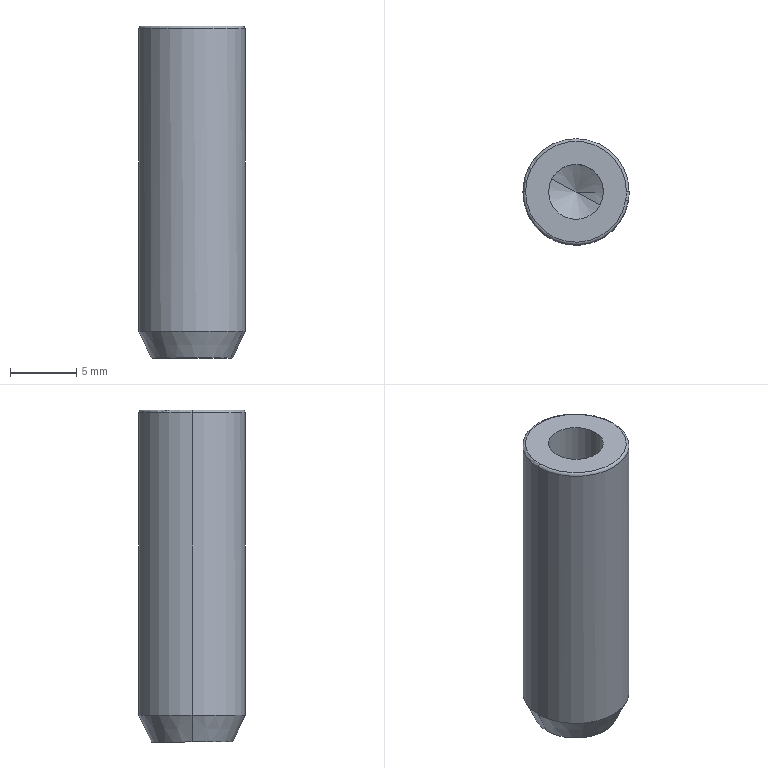Part | CATIA | 1 solid | 14 faces | box 8 x 8 x 25 mm | volume 1095 mm3 | cone 5 | cylinder 4 | torus 3 | plane 2 | commonest cylinder face diameters 4.134 x2 8 x2
STEP:
#1=CARTESIAN_POINT('',(0.,0.,13.807));
#2=VERTEX_POINT('',#1);
#3=CARTESIAN_POINT('',(-1.814,0.991,15.));
#4=VERTEX_POINT('',#3);
#5=CARTESIAN_POINT('',(-380004.396,207597.348,250013.807));
#6=DIRECTION('',(-0.76,0.4152,0.5));
#7=VECTOR('',#6,1.);
#8=LINE('',#5,#7);
#9=EDGE_CURVE('',#2,#4,#8,.T.);
#10=ORIENTED_EDGE('',*,*,#9,.T.);
#11=CARTESIAN_POINT('',(1.814,-0.991,15.));
#12=VERTEX_POINT('',#11);
#13=CARTESIAN_POINT('',(0.,0.,15.));
#14=DIRECTION('',(0.,0.,1.));
#15=AXIS2_PLACEMENT_3D('',#13,#14,$);
#16=CIRCLE('',#15,2.067);
#17=EDGE_CURVE('',#12,#4,#16,.F.);
#18=ORIENTED_EDGE('',*,*,#17,.F.);
#19=CARTESIAN_POINT('',(380004.396,-207597.348,250013.807));
#20=DIRECTION('',(0.76,-0.4152,0.5));
#21=VECTOR('',#20,1.);
#22=LINE('',#19,#21);
#23=EDGE_CURVE('',#2,#12,#22,.T.);
#24=ORIENTED_EDGE('',*,*,#23,.F.);
#25=EDGE_LOOP('',(#10,#18,#24));
#26=FACE_OUTER_BOUND('',#25,.T.);
#27=CARTESIAN_POINT('',(0.,0.,13.807));
#28=DIRECTION('',(0.,0.,1.));
#29=DIRECTION('',(-0.8776,0.4794,0.));
#30=AXIS2_PLACEMENT_3D('',#27,#28,#29);
#31=CONICAL_SURFACE('',#30,0.,1.047);
#32=ADVANCED_FACE('',(#26),#31,.F.);
#33=ORIENTED_EDGE('',*,*,#23,.T.);
#34=CARTESIAN_POINT('',(0.,0.,15.));
#35=DIRECTION('',(0.,0.,1.));
#36=AXIS2_PLACEMENT_3D('',#34,#35,$);
#37=CIRCLE('',#36,2.067);
#38=EDGE_CURVE('',#4,#12,#37,.F.);
#39=ORIENTED_EDGE('',*,*,#38,.F.);
#40=ORIENTED_EDGE('',*,*,#9,.F.);
#41=EDGE_LOOP('',(#33,#39,#40));
#42=FACE_OUTER_BOUND('',#41,.T.);
#43=CARTESIAN_POINT('',(0.,0.,13.807));
#44=DIRECTION('',(0.,0.,1.));
#45=DIRECTION('',(0.8776,-0.4794,0.));
#46=AXIS2_PLACEMENT_3D('',#43,#44,#45);
#47=CONICAL_SURFACE('',#46,0.,1.047);
#48=ADVANCED_FACE('',(#42),#47,.F.);
#49=CARTESIAN_POINT('',(-1.814,0.991,25.));
#50=VERTEX_POINT('',#49);
#51=CARTESIAN_POINT('',(1.814,-0.991,25.));
#52=VERTEX_POINT('',#51);
#53=CARTESIAN_POINT('',(0.,0.,25.));
#54=DIRECTION('',(0.,0.,-1.));
#55=AXIS2_PLACEMENT_3D('',#53,#54,$);
#56=CIRCLE('',#55,2.067);
#57=EDGE_CURVE('',#50,#52,#56,.F.);
#58=ORIENTED_EDGE('',*,*,#57,.T.);
#59=CARTESIAN_POINT('',(1.814,-0.991,24.9));
#60=DIRECTION('',(0.,0.,-1.));
#61=VECTOR('',#60,1.);
#62=LINE('',#59,#61);
#63=EDGE_CURVE('',#12,#52,#62,.F.);
#64=ORIENTED_EDGE('',*,*,#63,.F.);
#65=ORIENTED_EDGE('',*,*,#17,.T.);
#66=CARTESIAN_POINT('',(-1.814,0.991,24.9));
#67=DIRECTION('',(0.,0.,-1.));
#68=VECTOR('',#67,1.);
#69=LINE('',#66,#68);
#70=EDGE_CURVE('',#4,#50,#69,.F.);
#71=ORIENTED_EDGE('',*,*,#70,.T.);
#72=EDGE_LOOP('',(#58,#64,#65,#71));
#73=FACE_OUTER_BOUND('',#72,.T.);
#74=CARTESIAN_POINT('',(0.,0.,24.9));
#75=DIRECTION('',(0.,0.,-1.));
#76=DIRECTION('',(0.8776,-0.4794,0.));
#77=AXIS2_PLACEMENT_3D('',#74,#75,#76);
#78=CYLINDRICAL_SURFACE('',#77,2.067);
#79=ADVANCED_FACE('',(#73),#78,.F.);
#80=CARTESIAN_POINT('',(1.814,-0.991,25.));
#81=CARTESIAN_POINT('',(2.125,-0.4211,25.));
#82=CARTESIAN_POINT('',(2.213,0.271,25.));
#83=CARTESIAN_POINT('',(2.008,0.9675,25.));
#84=CARTESIAN_POINT('',(1.113,2.038,25.));
#85=CARTESIAN_POINT('',(-0.271,2.213,25.));
#86=CARTESIAN_POINT('',(-0.9675,2.008,25.));
#87=CARTESIAN_POINT('',(-1.503,1.561,25.));
#88=CARTESIAN_POINT('',(-1.814,0.991,25.));
#89=B_SPLINE_CURVE_WITH_KNOTS('',5,(#80,#81,#82,#83,#84,#85,#86,#87,#88),.UNSPECIFIED.,.F.,.U.,(6,3,6),(-3.247,0.,3.247),.UNSPECIFIED.);
#90=EDGE_CURVE('',#52,#50,#89,.T.);
#91=ORIENTED_EDGE('',*,*,#90,.T.);
#92=ORIENTED_EDGE('',*,*,#70,.F.);
#93=ORIENTED_EDGE('',*,*,#38,.T.);
#94=ORIENTED_EDGE('',*,*,#63,.T.);
#95=EDGE_LOOP('',(#91,#92,#93,#94));
#96=FACE_OUTER_BOUND('',#95,.T.);
#97=CARTESIAN_POINT('',(0.,0.,24.9));
#98=DIRECTION('',(0.,0.,-1.));
#99=DIRECTION('',(-0.8776,0.4794,0.));
#100=AXIS2_PLACEMENT_3D('',#97,#98,#99);
#101=CYLINDRICAL_SURFACE('',#100,2.067);
#102=ADVANCED_FACE('',(#96),#101,.F.);
#103=CARTESIAN_POINT('',(-3.8,0.000000372,25.));
#104=VERTEX_POINT('',#103);
#105=CARTESIAN_POINT('',(3.75,-0.6142,25.));
#106=VERTEX_POINT('',#105);
#107=CARTESIAN_POINT('',(0.,0.,25.));
#108=DIRECTION('',(0.,0.,1.));
#109=AXIS2_PLACEMENT_3D('',#107,#108,$);
#110=CIRCLE('',#109,3.8);
#111=EDGE_CURVE('',#104,#106,#110,.T.);
#112=ORIENTED_EDGE('',*,*,#111,.T.);
#113=CARTESIAN_POINT('',(3.8,0.,25.));
#114=VERTEX_POINT('',#113);
#115=CARTESIAN_POINT('',(0.,0.,25.));
#116=DIRECTION('',(0.,0.,1.));
#117=AXIS2_PLACEMENT_3D('',#115,#116,$);
#118=CIRCLE('',#117,3.8);
#119=EDGE_CURVE('',#106,#114,#118,.T.);
#120=ORIENTED_EDGE('',*,*,#119,.T.);
#121=CARTESIAN_POINT('',(0.,0.,25.));
#122=DIRECTION('',(0.,0.,1.));
#123=AXIS2_PLACEMENT_3D('',#121,#122,$);
#124=CIRCLE('',#123,3.8);
#125=EDGE_CURVE('',#114,#104,#124,.T.);
#126=ORIENTED_EDGE('',*,*,#125,.T.);
#127=EDGE_LOOP('',(#112,#120,#126));
#128=FACE_OUTER_BOUND('',#127,.T.);
#129=ORIENTED_EDGE('',*,*,#57,.F.);
#130=ORIENTED_EDGE('',*,*,#90,.F.);
#131=EDGE_LOOP('',(#129,#130));
#132=FACE_BOUND('',#131,.T.);
#133=CARTESIAN_POINT('',(0.,0.,25.));
#134=DIRECTION('',(0.,0.,1.));
#135=DIRECTION('',(1.,0.,0.));
#136=AXIS2_PLACEMENT_3D('',#133,#134,#135);
#137=PLANE('',#136);
#138=ADVANCED_FACE('',(#128,#132),#137,.T.);
#139=CARTESIAN_POINT('',(3.947,-0.6465,24.8));
#140=VERTEX_POINT('',#139);
#141=CARTESIAN_POINT('',(3.75,-0.6142,24.8));
#142=DIRECTION('',(-0.1616,-0.9869,0.));
#143=AXIS2_PLACEMENT_3D('',#141,#142,$);
#144=CIRCLE('',#143,0.2);
#145=EDGE_CURVE('',#140,#106,#144,.T.);
#146=ORIENTED_EDGE('',*,*,#145,.T.);
#147=ORIENTED_EDGE('',*,*,#111,.F.);
#148=CARTESIAN_POINT('',(-4.,0.,24.8));
#149=VERTEX_POINT('',#148);
#150=CARTESIAN_POINT('',(-3.8,0.,24.8));
#151=DIRECTION('',(0.,1.,0.));
#152=AXIS2_PLACEMENT_3D('',#150,#151,$);
#153=CIRCLE('',#152,0.2);
#154=EDGE_CURVE('',#104,#149,#153,.F.);
#155=ORIENTED_EDGE('',*,*,#154,.T.);
#156=CARTESIAN_POINT('',(0.,0.,24.8));
#157=DIRECTION('',(0.,0.,1.));
#158=AXIS2_PLACEMENT_3D('',#156,#157,$);
#159=CIRCLE('',#158,4.);
#160=EDGE_CURVE('',#149,#140,#159,.T.);
#161=ORIENTED_EDGE('',*,*,#160,.T.);
#162=EDGE_LOOP('',(#146,#147,#155,#161));
#163=FACE_OUTER_BOUND('',#162,.T.);
#164=CARTESIAN_POINT('',(0.,0.,24.8));
#165=DIRECTION('',(0.,0.,1.));
#166=DIRECTION('',(-0.9869,0.1616,0.));
#167=AXIS2_PLACEMENT_3D('',#164,#165,#166);
#168=TOROIDAL_SURFACE('',#167,3.8,0.2);
#169=ADVANCED_FACE('',(#163),#168,.T.);
#170=ORIENTED_EDGE('',*,*,#145,.F.);
#171=CARTESIAN_POINT('',(4.,0.,24.8));
#172=VERTEX_POINT('',#171);
#173=CARTESIAN_POINT('',(0.,0.,24.8));
#174=DIRECTION('',(0.,0.,1.));
#175=AXIS2_PLACEMENT_3D('',#173,#174,$);
#176=CIRCLE('',#175,4.);
#177=EDGE_CURVE('',#140,#172,#176,.T.);
#178=ORIENTED_EDGE('',*,*,#177,.T.);
#179=CARTESIAN_POINT('',(3.8,0.,24.8));
#180=DIRECTION('',(0.,-1.,0.));
#181=AXIS2_PLACEMENT_3D('',#179,#180,$);
#182=CIRCLE('',#181,0.2);
#183=EDGE_CURVE('',#114,#172,#182,.F.);
#184=ORIENTED_EDGE('',*,*,#183,.F.);
#185=ORIENTED_EDGE('',*,*,#119,.F.);
#186=EDGE_LOOP('',(#170,#178,#184,#185));
#187=FACE_OUTER_BOUND('',#186,.T.);
#188=CARTESIAN_POINT('',(0.,0.,24.8));
#189=DIRECTION('',(0.,0.,1.));
#190=DIRECTION('',(0.9869,-0.1616,0.));
#191=AXIS2_PLACEMENT_3D('',#188,#189,#190);
#192=TOROIDAL_SURFACE('',#191,3.8,0.2);
#193=ADVANCED_FACE('',(#187),#192,.T.);
#194=ORIENTED_EDGE('',*,*,#183,.T.);
#195=CARTESIAN_POINT('',(0.,0.,24.8));
#196=DIRECTION('',(0.,0.,1.));
#197=AXIS2_PLACEMENT_3D('',#195,#196,$);
#198=CIRCLE('',#197,4.);
#199=EDGE_CURVE('',#172,#149,#198,.T.);
#200=ORIENTED_EDGE('',*,*,#199,.T.);
#201=ORIENTED_EDGE('',*,*,#154,.F.);
#202=ORIENTED_EDGE('',*,*,#125,.F.);
#203=EDGE_LOOP('',(#194,#200,#201,#202));
#204=FACE_OUTER_BOUND('',#203,.T.);
#205=CARTESIAN_POINT('',(0.,0.,24.8));
#206=DIRECTION('',(0.,0.,1.));
#207=DIRECTION('',(1.,0.,0.));
#208=AXIS2_PLACEMENT_3D('',#205,#206,#207);
#209=TOROIDAL_SURFACE('',#208,3.8,0.2);
#210=ADVANCED_FACE('',(#204),#209,.T.);
#211=CARTESIAN_POINT('',(4.,0.,2.));
#212=VERTEX_POINT('',#211);
#213=CARTESIAN_POINT('',(4.,0.,12.5));
#214=DIRECTION('',(0.,0.,1.));
#215=VECTOR('',#214,1.);
#216=LINE('',#213,#215);
#217=EDGE_CURVE('',#212,#172,#216,.T.);
#218=ORIENTED_EDGE('',*,*,#217,.T.);
#219=ORIENTED_EDGE('',*,*,#177,.F.);
#220=ORIENTED_EDGE('',*,*,#160,.F.);
#221=CARTESIAN_POINT('',(-4.,0.,2.));
#222=VERTEX_POINT('',#221);
#223=CARTESIAN_POINT('',(-4.,0.,12.5));
#224=DIRECTION('',(0.,0.,1.));
#225=VECTOR('',#224,1.);
#226=LINE('',#223,#225);
#227=EDGE_CURVE('',#222,#149,#226,.T.);
#228=ORIENTED_EDGE('',*,*,#227,.F.);
#229=CARTESIAN_POINT('',(3.787,-1.287,2.));
#230=VERTEX_POINT('',#229);
#231=CARTESIAN_POINT('',(0.,0.,2.));
#232=DIRECTION('',(0.,0.,1.));
#233=AXIS2_PLACEMENT_3D('',#231,#232,$);
#234=CIRCLE('',#233,4.);
#235=EDGE_CURVE('',#222,#230,#234,.T.);
#236=ORIENTED_EDGE('',*,*,#235,.T.);
#237=CARTESIAN_POINT('',(0.,0.,2.));
#238=DIRECTION('',(0.,0.,1.));
#239=AXIS2_PLACEMENT_3D('',#237,#238,$);
#240=CIRCLE('',#239,4.);
#241=EDGE_CURVE('',#230,#212,#240,.T.);
#242=ORIENTED_EDGE('',*,*,#241,.T.);
#243=EDGE_LOOP('',(#218,#219,#220,#228,#236,#242));
#244=FACE_OUTER_BOUND('',#243,.T.);
#245=CARTESIAN_POINT('',(0.,0.,12.5));
#246=DIRECTION('',(0.,0.,1.));
#247=DIRECTION('',(-1.,0.,0.));
#248=AXIS2_PLACEMENT_3D('',#245,#246,#247);
#249=CYLINDRICAL_SURFACE('',#248,4.);
#250=ADVANCED_FACE('',(#244),#249,.T.);
#251=ORIENTED_EDGE('',*,*,#227,.T.);
#252=ORIENTED_EDGE('',*,*,#199,.F.);
#253=ORIENTED_EDGE('',*,*,#217,.F.);
#254=CARTESIAN_POINT('',(0.,0.,2.));
#255=DIRECTION('',(0.,0.,1.));
#256=AXIS2_PLACEMENT_3D('',#254,#255,$);
#257=CIRCLE('',#256,4.);
#258=EDGE_CURVE('',#212,#222,#257,.T.);
#259=ORIENTED_EDGE('',*,*,#258,.T.);
#260=EDGE_LOOP('',(#251,#252,#253,#259));
#261=FACE_OUTER_BOUND('',#260,.T.);
#262=CARTESIAN_POINT('',(0.,0.,12.5));
#263=DIRECTION('',(0.,0.,1.));
#264=DIRECTION('',(1.,0.,0.));
#265=AXIS2_PLACEMENT_3D('',#262,#263,#264);
#266=CYLINDRICAL_SURFACE('',#265,4.);
#267=ADVANCED_FACE('',(#261),#266,.T.);
#268=CARTESIAN_POINT('',(2.904,-0.9868,0.));
#269=VERTEX_POINT('',#268);
#270=CARTESIAN_POINT('',(200076.465,-67977.622,453147.315));
#271=DIRECTION('',(0.4002,-0.136,0.9063));
#272=VECTOR('',#271,1.);
#273=LINE('',#270,#272);
#274=EDGE_CURVE('',#269,#230,#273,.T.);
#275=ORIENTED_EDGE('',*,*,#274,.T.);
#276=ORIENTED_EDGE('',*,*,#235,.F.);
#277=CARTESIAN_POINT('',(-3.067,0.,0.));
#278=VERTEX_POINT('',#277);
#279=CARTESIAN_POINT('',(-3.067,0.000000238,0.));
#280=CARTESIAN_POINT('',(-3.378,0.000000159,0.6667));
#281=CARTESIAN_POINT('',(-3.689,0.000000415,1.333));
#282=CARTESIAN_POINT('',(-4.,0.000000311,2.));
#283=B_SPLINE_CURVE_WITH_KNOTS('',3,(#279,#280,#281,#282),.UNSPECIFIED.,.F.,.U.,(4,4),(0.,3.121),.UNSPECIFIED.);
#284=EDGE_CURVE('',#222,#278,#283,.F.);
#285=ORIENTED_EDGE('',*,*,#284,.T.);
#286=CARTESIAN_POINT('',(0.,0.,0.));
#287=DIRECTION('',(0.,0.,1.));
#288=AXIS2_PLACEMENT_3D('',#286,#287,$);
#289=CIRCLE('',#288,3.067);
#290=EDGE_CURVE('',#278,#269,#289,.T.);
#291=ORIENTED_EDGE('',*,*,#290,.T.);
#292=EDGE_LOOP('',(#275,#276,#285,#291));
#293=FACE_OUTER_BOUND('',#292,.T.);
#294=CARTESIAN_POINT('',(0.,0.,-6.578));
#295=DIRECTION('',(0.,0.,1.));
#296=DIRECTION('',(-0.9468,0.3217,0.));
#297=AXIS2_PLACEMENT_3D('',#294,#295,#296);
#298=CONICAL_SURFACE('',#297,0.,0.4363);
#299=ADVANCED_FACE('',(#293),#298,.T.);
#300=ORIENTED_EDGE('',*,*,#274,.F.);
#301=CARTESIAN_POINT('',(3.067,0.,0.));
#302=VERTEX_POINT('',#301);
#303=CARTESIAN_POINT('',(0.,0.,0.));
#304=DIRECTION('',(0.,0.,1.));
#305=AXIS2_PLACEMENT_3D('',#303,#304,$);
#306=CIRCLE('',#305,3.067);
#307=EDGE_CURVE('',#269,#302,#306,.T.);
#308=ORIENTED_EDGE('',*,*,#307,.T.);
#309=CARTESIAN_POINT('',(211309.131,0.000000151,453147.315));
#310=DIRECTION('',(0.4226,0.,0.9063));
#311=VECTOR('',#310,1.);
#312=LINE('',#309,#311);
#313=EDGE_CURVE('',#212,#302,#312,.F.);
#314=ORIENTED_EDGE('',*,*,#313,.F.);
#315=ORIENTED_EDGE('',*,*,#241,.F.);
#316=EDGE_LOOP('',(#300,#308,#314,#315));
#317=FACE_OUTER_BOUND('',#316,.T.);
#318=CARTESIAN_POINT('',(0.,0.,-6.578));
#319=DIRECTION('',(0.,0.,1.));
#320=DIRECTION('',(0.9468,-0.3217,0.));
#321=AXIS2_PLACEMENT_3D('',#318,#319,#320);
#322=CONICAL_SURFACE('',#321,0.,0.4363);
#323=ADVANCED_FACE('',(#317),#322,.T.);
#324=ORIENTED_EDGE('',*,*,#313,.T.);
#325=CARTESIAN_POINT('',(0.,0.,0.));
#326=DIRECTION('',(0.,0.,1.));
#327=AXIS2_PLACEMENT_3D('',#325,#326,$);
#328=CIRCLE('',#327,3.067);
#329=EDGE_CURVE('',#302,#278,#328,.T.);
#330=ORIENTED_EDGE('',*,*,#329,.T.);
#331=ORIENTED_EDGE('',*,*,#284,.F.);
#332=ORIENTED_EDGE('',*,*,#258,.F.);
#333=EDGE_LOOP('',(#324,#330,#331,#332));
#334=FACE_OUTER_BOUND('',#333,.T.);
#335=CARTESIAN_POINT('',(0.,0.,-6.578));
#336=DIRECTION('',(0.,0.,1.));
#337=DIRECTION('',(1.,0.,0.));
#338=AXIS2_PLACEMENT_3D('',#335,#336,#337);
#339=CONICAL_SURFACE('',#338,0.,0.4363);
#340=ADVANCED_FACE('',(#334),#339,.T.);
#341=ORIENTED_EDGE('',*,*,#329,.F.);
#342=ORIENTED_EDGE('',*,*,#307,.F.);
#343=ORIENTED_EDGE('',*,*,#290,.F.);
#344=EDGE_LOOP('',(#341,#342,#343));
#345=FACE_OUTER_BOUND('',#344,.T.);
#346=CARTESIAN_POINT('',(0.,0.,0.));
#347=DIRECTION('',(0.,0.,1.));
#348=DIRECTION('',(1.,0.,0.));
#349=AXIS2_PLACEMENT_3D('',#346,#347,#348);
#350=PLANE('',#349);
#351=ADVANCED_FACE('',(#345),#350,.F.);
#352=CLOSED_SHELL('',(#32,#48,#79,#102,#138,#169,#193,#210,#250,#267,#299,#323,#340,#351));
#353=MANIFOLD_SOLID_BREP('',#352);
#354=(LENGTH_UNIT()NAMED_UNIT(*)SI_UNIT(.MILLI.,.METRE.));
#355=UNCERTAINTY_MEASURE_WITH_UNIT(LENGTH_MEASURE(0.005),#354,'','');
#356=(NAMED_UNIT(*)PLANE_ANGLE_UNIT()SI_UNIT($,.RADIAN.));
#357=(NAMED_UNIT(*)SI_UNIT($,.STERADIAN.)SOLID_ANGLE_UNIT());
#358=(GEOMETRIC_REPRESENTATION_CONTEXT(3)GLOBAL_UNCERTAINTY_ASSIGNED_CONTEXT((#355))GLOBAL_UNIT_ASSIGNED_CONTEXT((#354,#356,#357))REPRESENTATION_CONTEXT('',''));
#359=ADVANCED_BREP_SHAPE_REPRESENTATION('',(#353),#358);